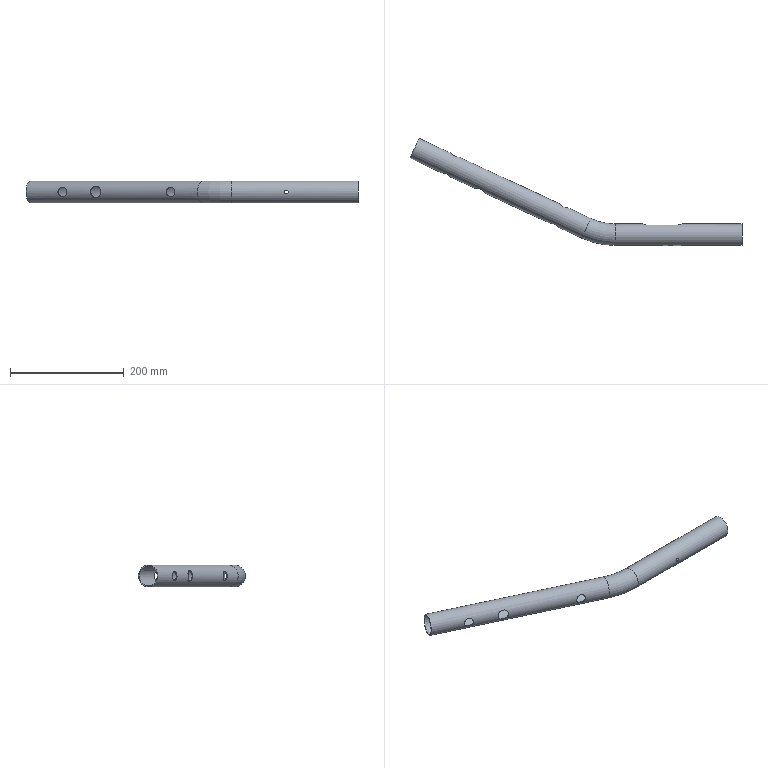Part | STEP file | 6151201R | 1 solid | 18 faces | box 584.322 x 188.458 x 38.1 mm | volume 101253 mm3 | cylinder 12 | plane 4 | torus 2 | commonest cylinder face diameters 17 x4 18 x2 35.1 x2 38.1 x2 7 x1 20 x1